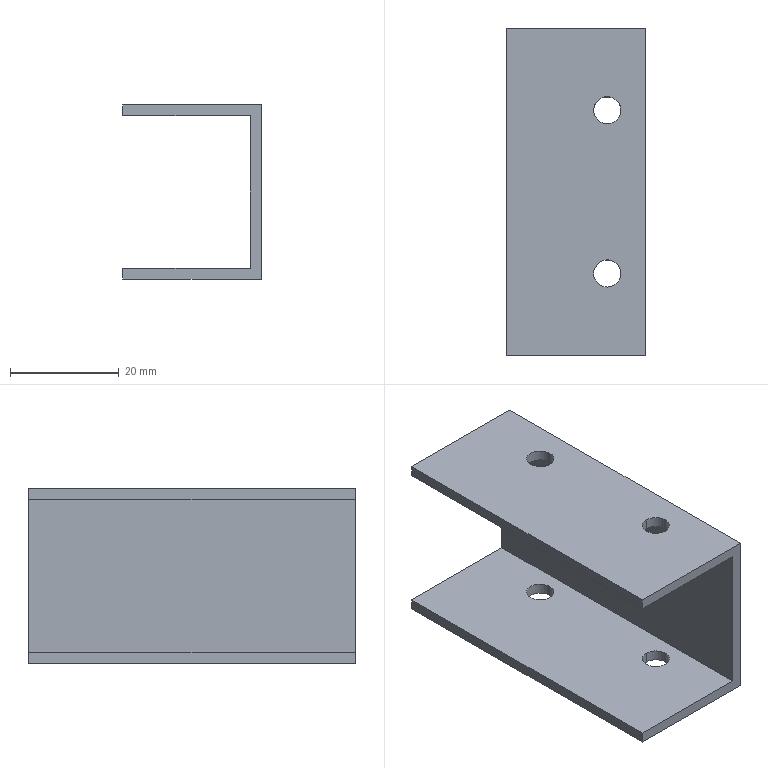Part | SolidWorks | features Cut 1, Extrusion 1, MirrorPattern 1 | 1 solid | 18 faces | box 25.474 x 60 x 32 mm | volume 9317 mm3 | plane 10 | cylinder 8 | commonest cylinder face diameters 5 x8
STEP:
#1=CARTESIAN_POINT('',(34.,37.5,0.));
#2=VERTEX_POINT('',#1);
#3=CARTESIAN_POINT('',(34.,32.5,0.));
#4=VERTEX_POINT('',#3);
#5=CARTESIAN_POINT('',(34.,35.,0.));
#6=DIRECTION('',(0.,0.,1.));
#7=DIRECTION('',(-1.,0.,0.));
#8=AXIS2_PLACEMENT_3D('',#5,#6,#7);
#9=CIRCLE('',#8,2.5);
#10=EDGE_CURVE('',#2,#4,#9,.T.);
#11=ORIENTED_EDGE('',*,*,#10,.F.);
#12=CARTESIAN_POINT('',(34.,37.5,2.));
#13=VERTEX_POINT('',#12);
#14=CARTESIAN_POINT('',(34.,37.5,-30.));
#15=DIRECTION('',(0.,0.,1.));
#16=VECTOR('',#15,1000.);
#17=LINE('',#14,#16);
#18=EDGE_CURVE('',#2,#13,#17,.T.);
#19=ORIENTED_EDGE('',*,*,#18,.T.);
#20=CARTESIAN_POINT('',(34.,32.5,2.));
#21=VERTEX_POINT('',#20);
#22=CARTESIAN_POINT('',(34.,35.,2.));
#23=DIRECTION('',(0.,0.,-1.));
#24=DIRECTION('',(1.,0.,0.));
#25=AXIS2_PLACEMENT_3D('',#22,#23,#24);
#26=CIRCLE('',#25,2.5);
#27=EDGE_CURVE('',#21,#13,#26,.T.);
#28=ORIENTED_EDGE('',*,*,#27,.F.);
#29=CARTESIAN_POINT('',(34.,32.5,-30.));
#30=DIRECTION('',(0.,0.,1.));
#31=VECTOR('',#30,1000.);
#32=LINE('',#29,#31);
#33=EDGE_CURVE('',#4,#21,#32,.T.);
#34=ORIENTED_EDGE('',*,*,#33,.F.);
#35=EDGE_LOOP('',(#11,#19,#28,#34));
#36=FACE_OUTER_BOUND('',#35,.T.);
#37=CARTESIAN_POINT('',(34.,35.,-30.));
#38=DIRECTION('',(0.,0.,1.));
#39=DIRECTION('',(0.,-1.,0.));
#40=AXIS2_PLACEMENT_3D('',#37,#38,#39);
#41=CYLINDRICAL_SURFACE('',#40,2.5);
#42=ADVANCED_FACE('',(#36),#41,.F.);
#43=CARTESIAN_POINT('',(34.,32.5,-30.));
#44=VERTEX_POINT('',#43);
#45=CARTESIAN_POINT('',(34.,37.5,-30.));
#46=VERTEX_POINT('',#45);
#47=CARTESIAN_POINT('',(34.,35.,-30.));
#48=DIRECTION('',(0.,0.,-1.));
#49=DIRECTION('',(1.,0.,0.));
#50=AXIS2_PLACEMENT_3D('',#47,#48,#49);
#51=CIRCLE('',#50,2.5);
#52=EDGE_CURVE('',#44,#46,#51,.T.);
#53=ORIENTED_EDGE('',*,*,#52,.T.);
#54=CARTESIAN_POINT('',(34.,37.5,-28.));
#55=VERTEX_POINT('',#54);
#56=CARTESIAN_POINT('',(34.,37.5,-30.));
#57=DIRECTION('',(0.,0.,1.));
#58=VECTOR('',#57,1000.);
#59=LINE('',#56,#58);
#60=EDGE_CURVE('',#46,#55,#59,.T.);
#61=ORIENTED_EDGE('',*,*,#60,.T.);
#62=CARTESIAN_POINT('',(34.,32.5,-28.));
#63=VERTEX_POINT('',#62);
#64=CARTESIAN_POINT('',(34.,35.,-28.));
#65=DIRECTION('',(0.,0.,-1.));
#66=DIRECTION('',(1.,0.,0.));
#67=AXIS2_PLACEMENT_3D('',#64,#65,#66);
#68=CIRCLE('',#67,2.5);
#69=EDGE_CURVE('',#63,#55,#68,.T.);
#70=ORIENTED_EDGE('',*,*,#69,.F.);
#71=CARTESIAN_POINT('',(34.,32.5,-30.));
#72=DIRECTION('',(0.,0.,1.));
#73=VECTOR('',#72,1000.);
#74=LINE('',#71,#73);
#75=EDGE_CURVE('',#44,#63,#74,.T.);
#76=ORIENTED_EDGE('',*,*,#75,.F.);
#77=EDGE_LOOP('',(#53,#61,#70,#76));
#78=FACE_OUTER_BOUND('',#77,.T.);
#79=CARTESIAN_POINT('',(34.,35.,-30.));
#80=DIRECTION('',(0.,0.,1.));
#81=DIRECTION('',(0.,-1.,0.));
#82=AXIS2_PLACEMENT_3D('',#79,#80,#81);
#83=CYLINDRICAL_SURFACE('',#82,2.5);
#84=ADVANCED_FACE('',(#78),#83,.F.);
#85=CARTESIAN_POINT('',(36.5,65.,0.));
#86=VERTEX_POINT('',#85);
#87=CARTESIAN_POINT('',(31.5,65.,0.));
#88=VERTEX_POINT('',#87);
#89=CARTESIAN_POINT('',(34.,65.,0.));
#90=DIRECTION('',(0.,0.,-1.));
#91=DIRECTION('',(-1.,0.,0.));
#92=AXIS2_PLACEMENT_3D('',#89,#90,#91);
#93=CIRCLE('',#92,2.5);
#94=EDGE_CURVE('',#86,#88,#93,.T.);
#95=ORIENTED_EDGE('',*,*,#94,.T.);
#96=CARTESIAN_POINT('',(31.5,65.,2.));
#97=VERTEX_POINT('',#96);
#98=CARTESIAN_POINT('',(31.5,65.,-30.));
#99=DIRECTION('',(0.,0.,1.));
#100=VECTOR('',#99,1000.);
#101=LINE('',#98,#100);
#102=EDGE_CURVE('',#88,#97,#101,.T.);
#103=ORIENTED_EDGE('',*,*,#102,.T.);
#104=CARTESIAN_POINT('',(36.5,65.,2.));
#105=VERTEX_POINT('',#104);
#106=CARTESIAN_POINT('',(34.,65.,2.));
#107=DIRECTION('',(0.,0.,1.));
#108=DIRECTION('',(1.,0.,0.));
#109=AXIS2_PLACEMENT_3D('',#106,#107,#108);
#110=CIRCLE('',#109,2.5);
#111=EDGE_CURVE('',#97,#105,#110,.T.);
#112=ORIENTED_EDGE('',*,*,#111,.T.);
#113=CARTESIAN_POINT('',(36.5,65.,-30.));
#114=DIRECTION('',(0.,0.,1.));
#115=VECTOR('',#114,1000.);
#116=LINE('',#113,#115);
#117=EDGE_CURVE('',#86,#105,#116,.T.);
#118=ORIENTED_EDGE('',*,*,#117,.F.);
#119=EDGE_LOOP('',(#95,#103,#112,#118));
#120=FACE_OUTER_BOUND('',#119,.T.);
#121=CARTESIAN_POINT('',(34.,65.,-30.));
#122=DIRECTION('',(0.,0.,1.));
#123=DIRECTION('',(1.,0.,0.));
#124=AXIS2_PLACEMENT_3D('',#121,#122,#123);
#125=CYLINDRICAL_SURFACE('',#124,2.5);
#126=ADVANCED_FACE('',(#120),#125,.F.);
#127=CARTESIAN_POINT('',(31.5,65.,-30.));
#128=VERTEX_POINT('',#127);
#129=CARTESIAN_POINT('',(36.5,65.,-30.));
#130=VERTEX_POINT('',#129);
#131=CARTESIAN_POINT('',(34.,65.,-30.));
#132=DIRECTION('',(0.,0.,1.));
#133=DIRECTION('',(1.,0.,0.));
#134=AXIS2_PLACEMENT_3D('',#131,#132,#133);
#135=CIRCLE('',#134,2.5);
#136=EDGE_CURVE('',#128,#130,#135,.T.);
#137=ORIENTED_EDGE('',*,*,#136,.F.);
#138=CARTESIAN_POINT('',(31.5,65.,-28.));
#139=VERTEX_POINT('',#138);
#140=CARTESIAN_POINT('',(31.5,65.,-30.));
#141=DIRECTION('',(0.,0.,1.));
#142=VECTOR('',#141,1000.);
#143=LINE('',#140,#142);
#144=EDGE_CURVE('',#128,#139,#143,.T.);
#145=ORIENTED_EDGE('',*,*,#144,.T.);
#146=CARTESIAN_POINT('',(36.5,65.,-28.));
#147=VERTEX_POINT('',#146);
#148=CARTESIAN_POINT('',(34.,65.,-28.));
#149=DIRECTION('',(0.,0.,1.));
#150=DIRECTION('',(1.,0.,0.));
#151=AXIS2_PLACEMENT_3D('',#148,#149,#150);
#152=CIRCLE('',#151,2.5);
#153=EDGE_CURVE('',#139,#147,#152,.T.);
#154=ORIENTED_EDGE('',*,*,#153,.T.);
#155=CARTESIAN_POINT('',(36.5,65.,-30.));
#156=DIRECTION('',(0.,0.,1.));
#157=VECTOR('',#156,1000.);
#158=LINE('',#155,#157);
#159=EDGE_CURVE('',#130,#147,#158,.T.);
#160=ORIENTED_EDGE('',*,*,#159,.F.);
#161=EDGE_LOOP('',(#137,#145,#154,#160));
#162=FACE_OUTER_BOUND('',#161,.T.);
#163=CARTESIAN_POINT('',(34.,65.,-30.));
#164=DIRECTION('',(0.,0.,1.));
#165=DIRECTION('',(1.,0.,0.));
#166=AXIS2_PLACEMENT_3D('',#163,#164,#165);
#167=CYLINDRICAL_SURFACE('',#166,2.5);
#168=ADVANCED_FACE('',(#162),#167,.F.);
#169=CARTESIAN_POINT('',(39.,80.,-28.));
#170=VERTEX_POINT('',#169);
#171=CARTESIAN_POINT('',(39.,20.,-28.));
#172=VERTEX_POINT('',#171);
#173=CARTESIAN_POINT('',(39.,80.,-28.));
#174=DIRECTION('',(0.,-1.,0.));
#175=VECTOR('',#174,1000.);
#176=LINE('',#173,#175);
#177=EDGE_CURVE('',#170,#172,#176,.T.);
#178=ORIENTED_EDGE('',*,*,#177,.T.);
#179=CARTESIAN_POINT('',(39.,20.,0.));
#180=VERTEX_POINT('',#179);
#181=CARTESIAN_POINT('',(39.,20.,0.));
#182=DIRECTION('',(0.,0.,-1.));
#183=VECTOR('',#182,1000.);
#184=LINE('',#181,#183);
#185=EDGE_CURVE('',#180,#172,#184,.T.);
#186=ORIENTED_EDGE('',*,*,#185,.F.);
#187=CARTESIAN_POINT('',(39.,80.,0.));
#188=VERTEX_POINT('',#187);
#189=CARTESIAN_POINT('',(39.,80.,0.));
#190=DIRECTION('',(0.,-1.,0.));
#191=VECTOR('',#190,1000.);
#192=LINE('',#189,#191);
#193=EDGE_CURVE('',#188,#180,#192,.T.);
#194=ORIENTED_EDGE('',*,*,#193,.F.);
#195=CARTESIAN_POINT('',(39.,80.,0.));
#196=DIRECTION('',(0.,0.,-1.));
#197=VECTOR('',#196,1000.);
#198=LINE('',#195,#197);
#199=EDGE_CURVE('',#188,#170,#198,.T.);
#200=ORIENTED_EDGE('',*,*,#199,.T.);
#201=EDGE_LOOP('',(#178,#186,#194,#200));
#202=FACE_OUTER_BOUND('',#201,.T.);
#203=CARTESIAN_POINT('',(39.,80.,0.));
#204=DIRECTION('',(-1.,0.,0.));
#205=DIRECTION('',(0.,0.,1.));
#206=AXIS2_PLACEMENT_3D('',#203,#204,#205);
#207=PLANE('',#206);
#208=ADVANCED_FACE('',(#202),#207,.T.);
#209=CARTESIAN_POINT('',(34.,35.,0.));
#210=DIRECTION('',(0.,0.,1.));
#211=DIRECTION('',(-1.,0.,0.));
#212=AXIS2_PLACEMENT_3D('',#209,#210,#211);
#213=CIRCLE('',#212,2.5);
#214=EDGE_CURVE('',#4,#2,#213,.T.);
#215=ORIENTED_EDGE('',*,*,#214,.T.);
#216=ORIENTED_EDGE('',*,*,#10,.T.);
#217=EDGE_LOOP('',(#215,#216));
#218=FACE_BOUND('',#217,.T.);
#219=ORIENTED_EDGE('',*,*,#94,.F.);
#220=CARTESIAN_POINT('',(34.,65.,0.));
#221=DIRECTION('',(0.,0.,-1.));
#222=DIRECTION('',(-1.,0.,0.));
#223=AXIS2_PLACEMENT_3D('',#220,#221,#222);
#224=CIRCLE('',#223,2.5);
#225=EDGE_CURVE('',#88,#86,#224,.T.);
#226=ORIENTED_EDGE('',*,*,#225,.F.);
#227=EDGE_LOOP('',(#219,#226));
#228=FACE_BOUND('',#227,.T.);
#229=ORIENTED_EDGE('',*,*,#193,.T.);
#230=CARTESIAN_POINT('',(15.526,20.,0.));
#231=VERTEX_POINT('',#230);
#232=CARTESIAN_POINT('',(15.526,20.,0.));
#233=DIRECTION('',(1.,0.,0.));
#234=VECTOR('',#233,1000.);
#235=LINE('',#232,#234);
#236=EDGE_CURVE('',#231,#180,#235,.T.);
#237=ORIENTED_EDGE('',*,*,#236,.F.);
#238=CARTESIAN_POINT('',(15.526,80.,0.));
#239=VERTEX_POINT('',#238);
#240=CARTESIAN_POINT('',(15.526,80.,0.));
#241=DIRECTION('',(0.,-1.,0.));
#242=VECTOR('',#241,1000.);
#243=LINE('',#240,#242);
#244=EDGE_CURVE('',#239,#231,#243,.T.);
#245=ORIENTED_EDGE('',*,*,#244,.F.);
#246=CARTESIAN_POINT('',(15.526,80.,0.));
#247=DIRECTION('',(1.,0.,0.));
#248=VECTOR('',#247,1000.);
#249=LINE('',#246,#248);
#250=EDGE_CURVE('',#239,#188,#249,.T.);
#251=ORIENTED_EDGE('',*,*,#250,.T.);
#252=EDGE_LOOP('',(#229,#237,#245,#251));
#253=FACE_OUTER_BOUND('',#252,.T.);
#254=CARTESIAN_POINT('',(15.526,80.,0.));
#255=DIRECTION('',(0.,0.,-1.));
#256=DIRECTION('',(-1.,0.,0.));
#257=AXIS2_PLACEMENT_3D('',#254,#255,#256);
#258=PLANE('',#257);
#259=ADVANCED_FACE('',(#218,#228,#253),#258,.T.);
#260=ORIENTED_EDGE('',*,*,#244,.T.);
#261=CARTESIAN_POINT('',(15.526,20.,2.));
#262=VERTEX_POINT('',#261);
#263=CARTESIAN_POINT('',(15.526,20.,2.));
#264=DIRECTION('',(0.,0.,-1.));
#265=VECTOR('',#264,1000.);
#266=LINE('',#263,#265);
#267=EDGE_CURVE('',#262,#231,#266,.T.);
#268=ORIENTED_EDGE('',*,*,#267,.F.);
#269=CARTESIAN_POINT('',(15.526,80.,2.));
#270=VERTEX_POINT('',#269);
#271=CARTESIAN_POINT('',(15.526,80.,2.));
#272=DIRECTION('',(0.,-1.,0.));
#273=VECTOR('',#272,1000.);
#274=LINE('',#271,#273);
#275=EDGE_CURVE('',#270,#262,#274,.T.);
#276=ORIENTED_EDGE('',*,*,#275,.F.);
#277=CARTESIAN_POINT('',(15.526,80.,2.));
#278=DIRECTION('',(0.,0.,-1.));
#279=VECTOR('',#278,1000.);
#280=LINE('',#277,#279);
#281=EDGE_CURVE('',#270,#239,#280,.T.);
#282=ORIENTED_EDGE('',*,*,#281,.T.);
#283=EDGE_LOOP('',(#260,#268,#276,#282));
#284=FACE_OUTER_BOUND('',#283,.T.);
#285=CARTESIAN_POINT('',(15.526,80.,2.));
#286=DIRECTION('',(-1.,0.,0.));
#287=DIRECTION('',(0.,0.,1.));
#288=AXIS2_PLACEMENT_3D('',#285,#286,#287);
#289=PLANE('',#288);
#290=ADVANCED_FACE('',(#284),#289,.T.);
#291=ORIENTED_EDGE('',*,*,#27,.T.);
#292=CARTESIAN_POINT('',(34.,35.,2.));
#293=DIRECTION('',(0.,0.,-1.));
#294=DIRECTION('',(1.,0.,0.));
#295=AXIS2_PLACEMENT_3D('',#292,#293,#294);
#296=CIRCLE('',#295,2.5);
#297=EDGE_CURVE('',#13,#21,#296,.T.);
#298=ORIENTED_EDGE('',*,*,#297,.T.);
#299=EDGE_LOOP('',(#291,#298));
#300=FACE_BOUND('',#299,.T.);
#301=CARTESIAN_POINT('',(34.,65.,2.));
#302=DIRECTION('',(0.,0.,1.));
#303=DIRECTION('',(1.,0.,0.));
#304=AXIS2_PLACEMENT_3D('',#301,#302,#303);
#305=CIRCLE('',#304,2.5);
#306=EDGE_CURVE('',#105,#97,#305,.T.);
#307=ORIENTED_EDGE('',*,*,#306,.F.);
#308=ORIENTED_EDGE('',*,*,#111,.F.);
#309=EDGE_LOOP('',(#307,#308));
#310=FACE_BOUND('',#309,.T.);
#311=ORIENTED_EDGE('',*,*,#275,.T.);
#312=CARTESIAN_POINT('',(41.,20.,2.));
#313=VERTEX_POINT('',#312);
#314=CARTESIAN_POINT('',(41.,20.,2.));
#315=DIRECTION('',(-1.,0.,0.));
#316=VECTOR('',#315,1000.);
#317=LINE('',#314,#316);
#318=EDGE_CURVE('',#313,#262,#317,.T.);
#319=ORIENTED_EDGE('',*,*,#318,.F.);
#320=CARTESIAN_POINT('',(41.,80.,2.));
#321=VERTEX_POINT('',#320);
#322=CARTESIAN_POINT('',(41.,80.,2.));
#323=DIRECTION('',(0.,-1.,0.));
#324=VECTOR('',#323,1000.);
#325=LINE('',#322,#324);
#326=EDGE_CURVE('',#321,#313,#325,.T.);
#327=ORIENTED_EDGE('',*,*,#326,.F.);
#328=CARTESIAN_POINT('',(41.,80.,2.));
#329=DIRECTION('',(-1.,0.,0.));
#330=VECTOR('',#329,1000.);
#331=LINE('',#328,#330);
#332=EDGE_CURVE('',#321,#270,#331,.T.);
#333=ORIENTED_EDGE('',*,*,#332,.T.);
#334=EDGE_LOOP('',(#311,#319,#327,#333));
#335=FACE_OUTER_BOUND('',#334,.T.);
#336=CARTESIAN_POINT('',(41.,80.,2.));
#337=DIRECTION('',(0.,0.,1.));
#338=DIRECTION('',(1.,0.,0.));
#339=AXIS2_PLACEMENT_3D('',#336,#337,#338);
#340=PLANE('',#339);
#341=ADVANCED_FACE('',(#300,#310,#335),#340,.T.);
#342=ORIENTED_EDGE('',*,*,#326,.T.);
#343=CARTESIAN_POINT('',(41.,20.,-30.));
#344=VERTEX_POINT('',#343);
#345=CARTESIAN_POINT('',(41.,20.,-30.));
#346=DIRECTION('',(0.,0.,1.));
#347=VECTOR('',#346,1000.);
#348=LINE('',#345,#347);
#349=EDGE_CURVE('',#344,#313,#348,.T.);
#350=ORIENTED_EDGE('',*,*,#349,.F.);
#351=CARTESIAN_POINT('',(41.,80.,-30.));
#352=VERTEX_POINT('',#351);
#353=CARTESIAN_POINT('',(41.,80.,-30.));
#354=DIRECTION('',(0.,-1.,0.));
#355=VECTOR('',#354,1000.);
#356=LINE('',#353,#355);
#357=EDGE_CURVE('',#352,#344,#356,.T.);
#358=ORIENTED_EDGE('',*,*,#357,.F.);
#359=CARTESIAN_POINT('',(41.,80.,-30.));
#360=DIRECTION('',(0.,0.,1.));
#361=VECTOR('',#360,1000.);
#362=LINE('',#359,#361);
#363=EDGE_CURVE('',#352,#321,#362,.T.);
#364=ORIENTED_EDGE('',*,*,#363,.T.);
#365=EDGE_LOOP('',(#342,#350,#358,#364));
#366=FACE_OUTER_BOUND('',#365,.T.);
#367=CARTESIAN_POINT('',(41.,80.,-30.));
#368=DIRECTION('',(1.,0.,0.));
#369=DIRECTION('',(0.,0.,-1.));
#370=AXIS2_PLACEMENT_3D('',#367,#368,#369);
#371=PLANE('',#370);
#372=ADVANCED_FACE('',(#366),#371,.T.);
#373=ORIENTED_EDGE('',*,*,#52,.F.);
#374=CARTESIAN_POINT('',(34.,35.,-30.));
#375=DIRECTION('',(0.,0.,-1.));
#376=DIRECTION('',(1.,0.,0.));
#377=AXIS2_PLACEMENT_3D('',#374,#375,#376);
#378=CIRCLE('',#377,2.5);
#379=EDGE_CURVE('',#46,#44,#378,.T.);
#380=ORIENTED_EDGE('',*,*,#379,.F.);
#381=EDGE_LOOP('',(#373,#380));
#382=FACE_BOUND('',#381,.T.);
#383=CARTESIAN_POINT('',(34.,65.,-30.));
#384=DIRECTION('',(0.,0.,1.));
#385=DIRECTION('',(1.,0.,0.));
#386=AXIS2_PLACEMENT_3D('',#383,#384,#385);
#387=CIRCLE('',#386,2.5);
#388=EDGE_CURVE('',#130,#128,#387,.T.);
#389=ORIENTED_EDGE('',*,*,#388,.T.);
#390=ORIENTED_EDGE('',*,*,#136,.T.);
#391=EDGE_LOOP('',(#389,#390));
#392=FACE_BOUND('',#391,.T.);
#393=ORIENTED_EDGE('',*,*,#357,.T.);
#394=CARTESIAN_POINT('',(15.526,20.,-30.));
#395=VERTEX_POINT('',#394);
#396=CARTESIAN_POINT('',(15.526,20.,-30.));
#397=DIRECTION('',(1.,0.,0.));
#398=VECTOR('',#397,1000.);
#399=LINE('',#396,#398);
#400=EDGE_CURVE('',#395,#344,#399,.T.);
#401=ORIENTED_EDGE('',*,*,#400,.F.);
#402=CARTESIAN_POINT('',(15.526,80.,-30.));
#403=VERTEX_POINT('',#402);
#404=CARTESIAN_POINT('',(15.526,80.,-30.));
#405=DIRECTION('',(0.,-1.,0.));
#406=VECTOR('',#405,1000.);
#407=LINE('',#404,#406);
#408=EDGE_CURVE('',#403,#395,#407,.T.);
#409=ORIENTED_EDGE('',*,*,#408,.F.);
#410=CARTESIAN_POINT('',(15.526,80.,-30.));
#411=DIRECTION('',(1.,0.,0.));
#412=VECTOR('',#411,1000.);
#413=LINE('',#410,#412);
#414=EDGE_CURVE('',#403,#352,#413,.T.);
#415=ORIENTED_EDGE('',*,*,#414,.T.);
#416=EDGE_LOOP('',(#393,#401,#409,#415));
#417=FACE_OUTER_BOUND('',#416,.T.);
#418=CARTESIAN_POINT('',(15.526,80.,-30.));
#419=DIRECTION('',(0.,0.,-1.));
#420=DIRECTION('',(-1.,0.,0.));
#421=AXIS2_PLACEMENT_3D('',#418,#419,#420);
#422=PLANE('',#421);
#423=ADVANCED_FACE('',(#382,#392,#417),#422,.T.);
#424=ORIENTED_EDGE('',*,*,#408,.T.);
#425=CARTESIAN_POINT('',(15.526,20.,-28.));
#426=VERTEX_POINT('',#425);
#427=CARTESIAN_POINT('',(15.526,20.,-28.));
#428=DIRECTION('',(0.,0.,-1.));
#429=VECTOR('',#428,1000.);
#430=LINE('',#427,#429);
#431=EDGE_CURVE('',#426,#395,#430,.T.);
#432=ORIENTED_EDGE('',*,*,#431,.F.);
#433=CARTESIAN_POINT('',(15.526,80.,-28.));
#434=VERTEX_POINT('',#433);
#435=CARTESIAN_POINT('',(15.526,80.,-28.));
#436=DIRECTION('',(0.,-1.,0.));
#437=VECTOR('',#436,1000.);
#438=LINE('',#435,#437);
#439=EDGE_CURVE('',#434,#426,#438,.T.);
#440=ORIENTED_EDGE('',*,*,#439,.F.);
#441=CARTESIAN_POINT('',(15.526,80.,-28.));
#442=DIRECTION('',(0.,0.,-1.));
#443=VECTOR('',#442,1000.);
#444=LINE('',#441,#443);
#445=EDGE_CURVE('',#434,#403,#444,.T.);
#446=ORIENTED_EDGE('',*,*,#445,.T.);
#447=EDGE_LOOP('',(#424,#432,#440,#446));
#448=FACE_OUTER_BOUND('',#447,.T.);
#449=CARTESIAN_POINT('',(15.526,80.,-28.));
#450=DIRECTION('',(-1.,0.,0.));
#451=DIRECTION('',(0.,0.,1.));
#452=AXIS2_PLACEMENT_3D('',#449,#450,#451);
#453=PLANE('',#452);
#454=ADVANCED_FACE('',(#448),#453,.T.);
#455=ORIENTED_EDGE('',*,*,#69,.T.);
#456=CARTESIAN_POINT('',(34.,35.,-28.));
#457=DIRECTION('',(0.,0.,-1.));
#458=DIRECTION('',(1.,0.,0.));
#459=AXIS2_PLACEMENT_3D('',#456,#457,#458);
#460=CIRCLE('',#459,2.5);
#461=EDGE_CURVE('',#55,#63,#460,.T.);
#462=ORIENTED_EDGE('',*,*,#461,.T.);
#463=EDGE_LOOP('',(#455,#462));
#464=FACE_BOUND('',#463,.T.);
#465=CARTESIAN_POINT('',(34.,65.,-28.));
#466=DIRECTION('',(0.,0.,1.));
#467=DIRECTION('',(1.,0.,0.));
#468=AXIS2_PLACEMENT_3D('',#465,#466,#467);
#469=CIRCLE('',#468,2.5);
#470=EDGE_CURVE('',#147,#139,#469,.T.);
#471=ORIENTED_EDGE('',*,*,#470,.F.);
#472=ORIENTED_EDGE('',*,*,#153,.F.);
#473=EDGE_LOOP('',(#471,#472));
#474=FACE_BOUND('',#473,.T.);
#475=ORIENTED_EDGE('',*,*,#439,.T.);
#476=CARTESIAN_POINT('',(39.,20.,-28.));
#477=DIRECTION('',(-1.,0.,0.));
#478=VECTOR('',#477,1000.);
#479=LINE('',#476,#478);
#480=EDGE_CURVE('',#172,#426,#479,.T.);
#481=ORIENTED_EDGE('',*,*,#480,.F.);
#482=ORIENTED_EDGE('',*,*,#177,.F.);
#483=CARTESIAN_POINT('',(39.,80.,-28.));
#484=DIRECTION('',(-1.,0.,0.));
#485=VECTOR('',#484,1000.);
#486=LINE('',#483,#485);
#487=EDGE_CURVE('',#170,#434,#486,.T.);
#488=ORIENTED_EDGE('',*,*,#487,.T.);
#489=EDGE_LOOP('',(#475,#481,#482,#488));
#490=FACE_OUTER_BOUND('',#489,.T.);
#491=CARTESIAN_POINT('',(39.,80.,-28.));
#492=DIRECTION('',(0.,0.,1.));
#493=DIRECTION('',(1.,0.,0.));
#494=AXIS2_PLACEMENT_3D('',#491,#492,#493);
#495=PLANE('',#494);
#496=ADVANCED_FACE('',(#464,#474,#490),#495,.T.);
#497=ORIENTED_EDGE('',*,*,#199,.F.);
#498=ORIENTED_EDGE('',*,*,#250,.F.);
#499=ORIENTED_EDGE('',*,*,#281,.F.);
#500=ORIENTED_EDGE('',*,*,#332,.F.);
#501=ORIENTED_EDGE('',*,*,#363,.F.);
#502=ORIENTED_EDGE('',*,*,#414,.F.);
#503=ORIENTED_EDGE('',*,*,#445,.F.);
#504=ORIENTED_EDGE('',*,*,#487,.F.);
#505=EDGE_LOOP('',(#497,#498,#499,#500,#501,#502,#503,#504));
#506=FACE_OUTER_BOUND('',#505,.T.);
#507=CARTESIAN_POINT('',(0.,80.,0.));
#508=DIRECTION('',(0.,1.,0.));
#509=DIRECTION('',(0.,0.,1.));
#510=AXIS2_PLACEMENT_3D('',#507,#508,#509);
#511=PLANE('',#510);
#512=ADVANCED_FACE('',(#506),#511,.T.);
#513=ORIENTED_EDGE('',*,*,#185,.T.);
#514=ORIENTED_EDGE('',*,*,#480,.T.);
#515=ORIENTED_EDGE('',*,*,#431,.T.);
#516=ORIENTED_EDGE('',*,*,#400,.T.);
#517=ORIENTED_EDGE('',*,*,#349,.T.);
#518=ORIENTED_EDGE('',*,*,#318,.T.);
#519=ORIENTED_EDGE('',*,*,#267,.T.);
#520=ORIENTED_EDGE('',*,*,#236,.T.);
#521=EDGE_LOOP('',(#513,#514,#515,#516,#517,#518,#519,#520));
#522=FACE_OUTER_BOUND('',#521,.T.);
#523=CARTESIAN_POINT('',(0.,20.,0.));
#524=DIRECTION('',(0.,1.,0.));
#525=DIRECTION('',(0.,0.,1.));
#526=AXIS2_PLACEMENT_3D('',#523,#524,#525);
#527=PLANE('',#526);
#528=ADVANCED_FACE('',(#522),#527,.F.);
#529=ORIENTED_EDGE('',*,*,#144,.F.);
#530=ORIENTED_EDGE('',*,*,#388,.F.);
#531=ORIENTED_EDGE('',*,*,#159,.T.);
#532=ORIENTED_EDGE('',*,*,#470,.T.);
#533=EDGE_LOOP('',(#529,#530,#531,#532));
#534=FACE_OUTER_BOUND('',#533,.T.);
#535=CARTESIAN_POINT('',(34.,65.,-30.));
#536=DIRECTION('',(0.,0.,1.));
#537=DIRECTION('',(1.,0.,0.));
#538=AXIS2_PLACEMENT_3D('',#535,#536,#537);
#539=CYLINDRICAL_SURFACE('',#538,2.5);
#540=ADVANCED_FACE('',(#534),#539,.F.);
#541=ORIENTED_EDGE('',*,*,#102,.F.);
#542=ORIENTED_EDGE('',*,*,#225,.T.);
#543=ORIENTED_EDGE('',*,*,#117,.T.);
#544=ORIENTED_EDGE('',*,*,#306,.T.);
#545=EDGE_LOOP('',(#541,#542,#543,#544));
#546=FACE_OUTER_BOUND('',#545,.T.);
#547=CARTESIAN_POINT('',(34.,65.,-30.));
#548=DIRECTION('',(0.,0.,1.));
#549=DIRECTION('',(1.,0.,0.));
#550=AXIS2_PLACEMENT_3D('',#547,#548,#549);
#551=CYLINDRICAL_SURFACE('',#550,2.5);
#552=ADVANCED_FACE('',(#546),#551,.F.);
#553=ORIENTED_EDGE('',*,*,#60,.F.);
#554=ORIENTED_EDGE('',*,*,#379,.T.);
#555=ORIENTED_EDGE('',*,*,#75,.T.);
#556=ORIENTED_EDGE('',*,*,#461,.F.);
#557=EDGE_LOOP('',(#553,#554,#555,#556));
#558=FACE_OUTER_BOUND('',#557,.T.);
#559=CARTESIAN_POINT('',(34.,35.,-30.));
#560=DIRECTION('',(0.,0.,1.));
#561=DIRECTION('',(0.,-1.,0.));
#562=AXIS2_PLACEMENT_3D('',#559,#560,#561);
#563=CYLINDRICAL_SURFACE('',#562,2.5);
#564=ADVANCED_FACE('',(#558),#563,.F.);
#565=ORIENTED_EDGE('',*,*,#18,.F.);
#566=ORIENTED_EDGE('',*,*,#214,.F.);
#567=ORIENTED_EDGE('',*,*,#33,.T.);
#568=ORIENTED_EDGE('',*,*,#297,.F.);
#569=EDGE_LOOP('',(#565,#566,#567,#568));
#570=FACE_OUTER_BOUND('',#569,.T.);
#571=CARTESIAN_POINT('',(34.,35.,-30.));
#572=DIRECTION('',(0.,0.,1.));
#573=DIRECTION('',(0.,-1.,0.));
#574=AXIS2_PLACEMENT_3D('',#571,#572,#573);
#575=CYLINDRICAL_SURFACE('',#574,2.5);
#576=ADVANCED_FACE('',(#570),#575,.F.);
#577=CLOSED_SHELL('',(#42,#84,#126,#168,#208,#259,#290,#341,#372,#423,#454,#496,#512,#528,#540,#552,#564,#576));
#578=MANIFOLD_SOLID_BREP('',#577);
#579=CARTESIAN_POINT('',(0.,0.,0.));
#580=DIRECTION('',(0.,0.,1.));
#581=DIRECTION('',(1.,0.,0.));
#582=AXIS2_PLACEMENT_3D('',#579,#580,#581);
#583=(LENGTH_UNIT()NAMED_UNIT(*)SI_UNIT(.MILLI.,.METRE.));
#584=UNCERTAINTY_MEASURE_WITH_UNIT(LENGTH_MEASURE(0.00001),#583,'','');
#585=(NAMED_UNIT(*)PLANE_ANGLE_UNIT()SI_UNIT($,.RADIAN.));
#586=(NAMED_UNIT(*)SI_UNIT($,.STERADIAN.)SOLID_ANGLE_UNIT());
#587=(GEOMETRIC_REPRESENTATION_CONTEXT(3)GLOBAL_UNCERTAINTY_ASSIGNED_CONTEXT((#584))GLOBAL_UNIT_ASSIGNED_CONTEXT((#583,#585,#586))REPRESENTATION_CONTEXT('',''));
#588=ADVANCED_BREP_SHAPE_REPRESENTATION('',(#578,#582),#587);